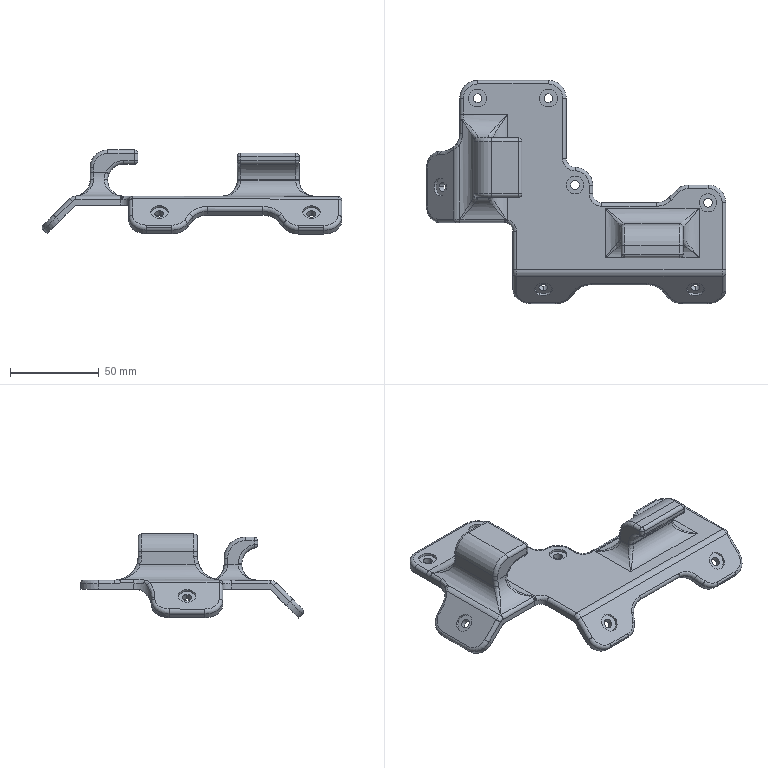Part | SolidWorks | features BaseBody 1 | 1 solid | 214 faces | box 168.933 x 125.849 x 47.457 mm | volume 88777 mm3 | cylinder 109 | plane 44 | torus 34 | spline 16 | sphere 11 | commonest cylinder face diameters 4 x45 10 x19 20 x16 5 x14 18 x8 1 x2